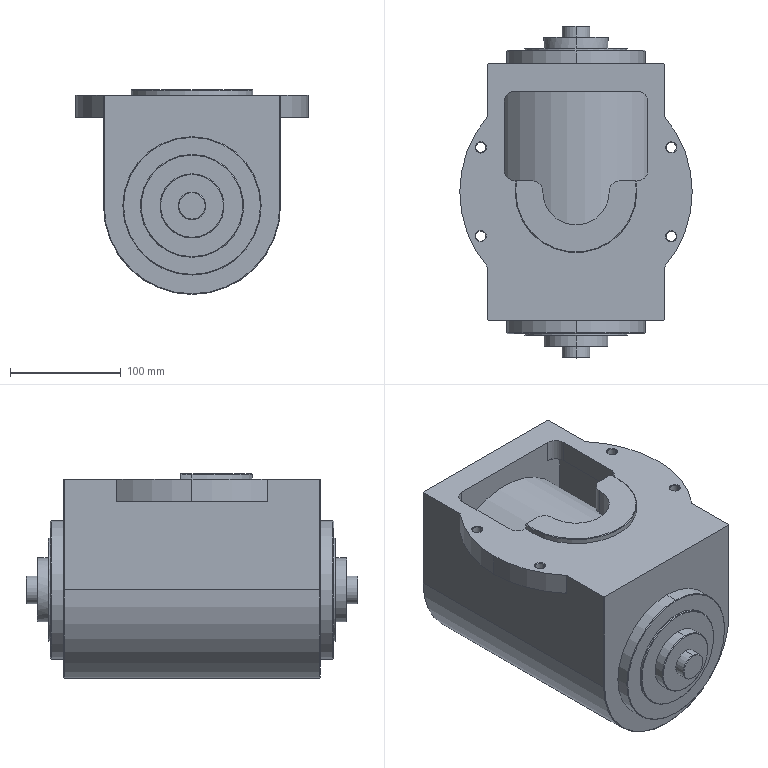Part | SolidWorks | features BaseBody 1 | 1 solid | 107 faces | box 210 x 300 x 185.1 mm | volume 5982188 mm3 | cylinder 40 | cone 38 | plane 29 | commonest cylinder face diameters 9 x8 20 x6 25 x4 58 x4 93 x4 125 x4